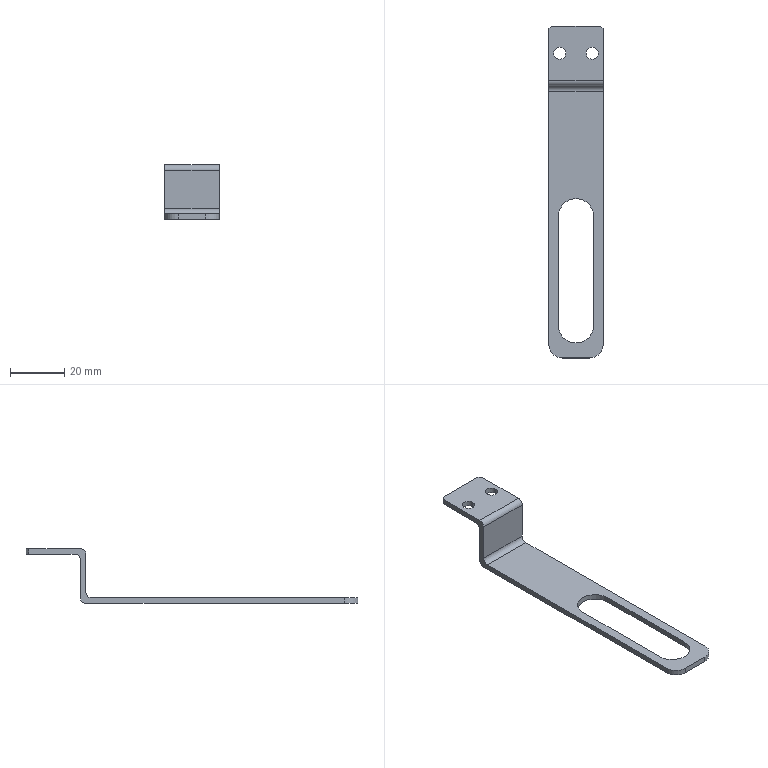Part | STEP file | Proximity Switch Bracket | 1 solid | 26 faces | box 20 x 122 x 20 mm | volume 4207 mm3 | plane 14 | cylinder 12 | commonest cylinder face diameters 4 x4 4.5 x4 10 x2 13 x2